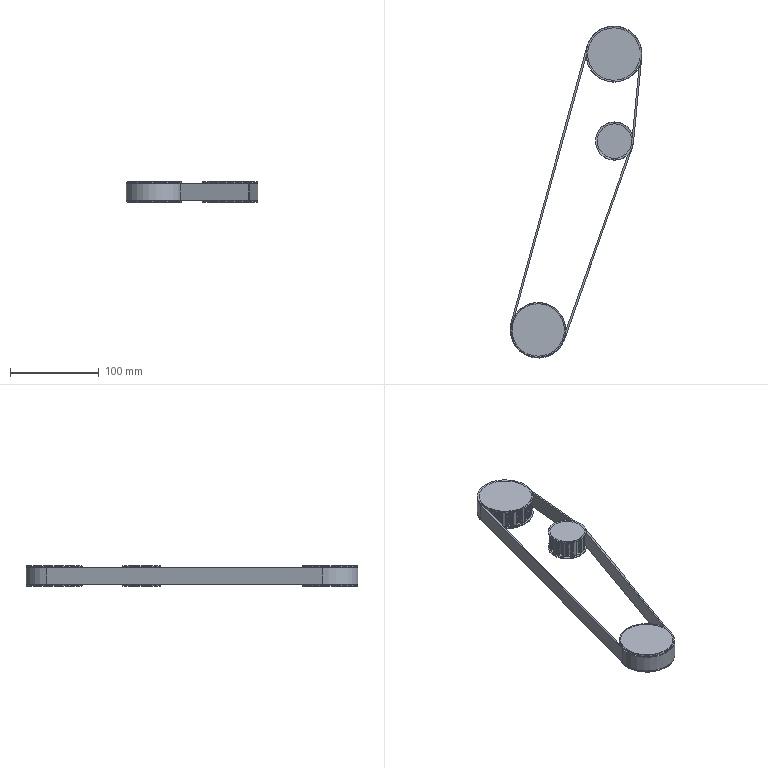Part | SolidWorks | 4 solids | 629 faces | box 148.838 x 374.646 x 23.437 mm | volume 174759 mm3 | cylinder 367 | plane 214 | cone 36 | torus 12 | commonest cylinder face diameters 3.2 x320 59.266 x32 39.054 x12 63.33 x2 43.118 x1